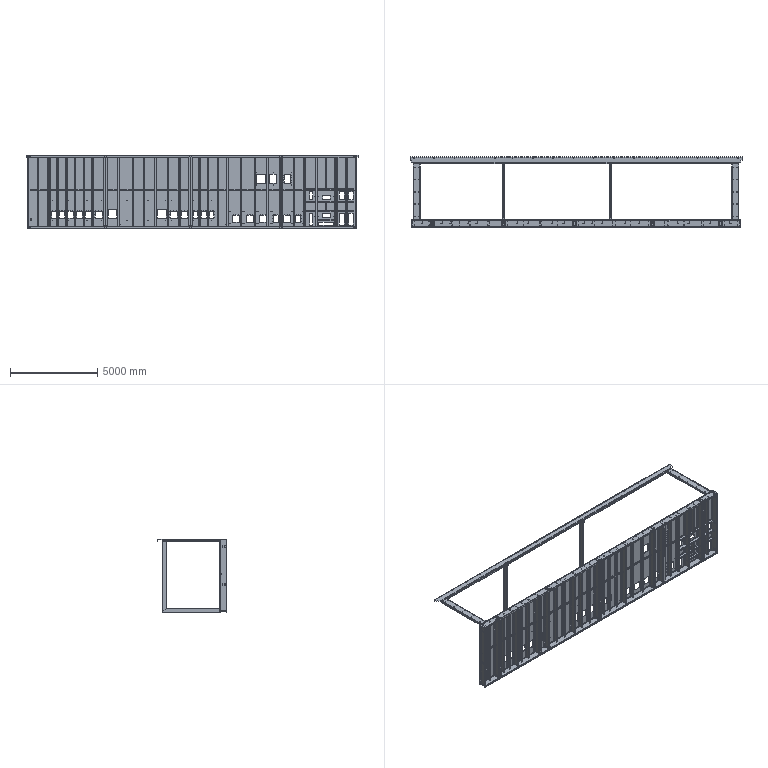Part | STEP file | TS-BASE01_default<by machining> | 141 solids | 3728 faces | volume 1776605339 mm3 | plane 1816 | cylinder 1792 | cone 120 | commonest cylinder face diameters 10 x608 24 x258 18 x120 21 x120 28 x120 11.5 x92